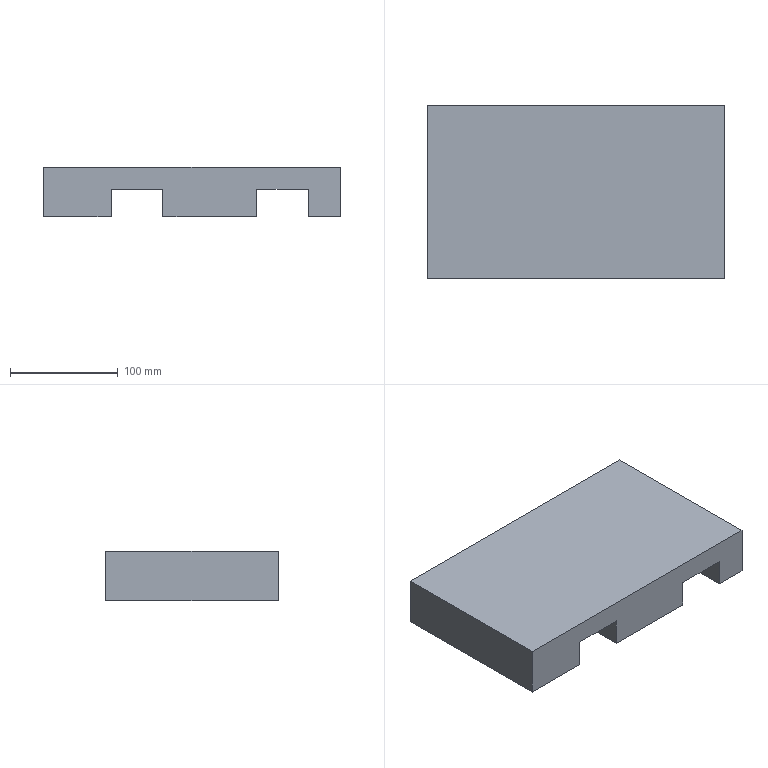Part | 1 solid | 14 faces | box 275.4 x 160 x 46 mm | volume 1635264 mm3 | plane 14
STEP:
#1=CARTESIAN_POINT('',(0.,0.,0.));
#2=DIRECTION('',(0.,0.,1.));
#3=DIRECTION('',(1.,0.,0.));
#4=AXIS2_PLACEMENT_3D('',#1,#2,#3);
#5=CARTESIAN_POINT('',(-116.3,226.5,-322.55));
#6=VERTEX_POINT('',#5);
#7=CARTESIAN_POINT('',(-116.3,226.5,-276.55));
#8=VERTEX_POINT('',#7);
#9=CARTESIAN_POINT('',(-116.3,226.5,-306.55));
#10=DIRECTION('',(0.,0.,1.));
#11=VECTOR('',#10,1.);
#12=LINE('',#9,#11);
#13=CARTESIAN_POINT('',(-116.3,386.5,-306.55));
#14=DIRECTION('',(1.,0.,0.));
#15=DIRECTION('',(0.,0.,-1.));
#16=AXIS2_PLACEMENT_3D('',#13,#14,#15);
#17=PLANE('',#16);
#18=CARTESIAN_POINT('',(0.,-160.));
#19=DIRECTION('',(-1.,0.));
#20=VECTOR('',#19,1.);
#21=LINE('',#18,#20);
#22=(GEOMETRIC_REPRESENTATION_CONTEXT(2)PARAMETRIC_REPRESENTATION_CONTEXT()REPRESENTATION_CONTEXT('',''));
#23=DEFINITIONAL_REPRESENTATION('',(#21),#22);
#24=PCURVE('',#17,#23);
#25=CARTESIAN_POINT('',(-287.5,226.5,-306.55));
#26=DIRECTION('',(0.,1.,0.));
#27=DIRECTION('',(0.,0.,-1.));
#28=AXIS2_PLACEMENT_3D('',#25,#26,#27);
#29=PLANE('',#28);
#30=CARTESIAN_POINT('',(0.,-171.2));
#31=DIRECTION('',(-1.,0.));
#32=VECTOR('',#31,1.);
#33=LINE('',#30,#32);
#34=(GEOMETRIC_REPRESENTATION_CONTEXT(2)PARAMETRIC_REPRESENTATION_CONTEXT()REPRESENTATION_CONTEXT('',''));
#35=DEFINITIONAL_REPRESENTATION('',(#33),#34);
#36=PCURVE('',#29,#35);
#37=SURFACE_CURVE('',#12,(#24,#36),.PCURVE_S1.);
#38=EDGE_CURVE('',#6,#8,#37,.T.);
#39=ORIENTED_EDGE('',*,*,#38,.F.);
#40=CARTESIAN_POINT('',(-116.3,386.5,-322.55));
#41=VERTEX_POINT('',#40);
#42=CARTESIAN_POINT('',(-116.3,386.5,-322.55));
#43=DIRECTION('',(0.,-1.,0.));
#44=VECTOR('',#43,1.);
#45=LINE('',#42,#44);
#46=CARTESIAN_POINT('',(16.,0.));
#47=DIRECTION('',(0.,-1.));
#48=VECTOR('',#47,1.);
#49=LINE('',#46,#48);
#50=(GEOMETRIC_REPRESENTATION_CONTEXT(2)PARAMETRIC_REPRESENTATION_CONTEXT()REPRESENTATION_CONTEXT('',''));
#51=DEFINITIONAL_REPRESENTATION('',(#49),#50);
#52=PCURVE('',#17,#51);
#53=CARTESIAN_POINT('',(-384.03,386.5,-322.55));
#54=DIRECTION('',(0.,0.,1.));
#55=DIRECTION('',(1.,0.,0.));
#56=AXIS2_PLACEMENT_3D('',#53,#54,#55);
#57=PLANE('',#56);
#58=CARTESIAN_POINT('',(267.73,0.));
#59=DIRECTION('',(0.,-1.));
#60=VECTOR('',#59,1.);
#61=LINE('',#58,#60);
#62=(GEOMETRIC_REPRESENTATION_CONTEXT(2)PARAMETRIC_REPRESENTATION_CONTEXT()REPRESENTATION_CONTEXT('',''));
#63=DEFINITIONAL_REPRESENTATION('',(#61),#62);
#64=PCURVE('',#57,#63);
#65=SURFACE_CURVE('',#45,(#52,#64),.PCURVE_S1.);
#66=EDGE_CURVE('',#41,#6,#65,.T.);
#67=ORIENTED_EDGE('',*,*,#66,.F.);
#68=CARTESIAN_POINT('',(-116.3,386.5,-276.55));
#69=VERTEX_POINT('',#68);
#70=CARTESIAN_POINT('',(-116.3,386.5,-306.55));
#71=DIRECTION('',(0.,0.,1.));
#72=VECTOR('',#71,1.);
#73=LINE('',#70,#72);
#74=CARTESIAN_POINT('',(0.,0.));
#75=DIRECTION('',(-1.,0.));
#76=VECTOR('',#75,1.);
#77=LINE('',#74,#76);
#78=(GEOMETRIC_REPRESENTATION_CONTEXT(2)PARAMETRIC_REPRESENTATION_CONTEXT()REPRESENTATION_CONTEXT('',''));
#79=DEFINITIONAL_REPRESENTATION('',(#77),#78);
#80=PCURVE('',#17,#79);
#81=CARTESIAN_POINT('',(-287.5,386.5,-306.55));
#82=DIRECTION('',(0.,1.,0.));
#83=DIRECTION('',(0.,0.,-1.));
#84=AXIS2_PLACEMENT_3D('',#81,#82,#83);
#85=PLANE('',#84);
#86=CARTESIAN_POINT('',(0.,-171.2));
#87=DIRECTION('',(-1.,0.));
#88=VECTOR('',#87,1.);
#89=LINE('',#86,#88);
#90=(GEOMETRIC_REPRESENTATION_CONTEXT(2)PARAMETRIC_REPRESENTATION_CONTEXT()REPRESENTATION_CONTEXT('',''));
#91=DEFINITIONAL_REPRESENTATION('',(#89),#90);
#92=PCURVE('',#85,#91);
#93=SURFACE_CURVE('',#73,(#80,#92),.PCURVE_S1.);
#94=EDGE_CURVE('',#41,#69,#93,.T.);
#95=ORIENTED_EDGE('',*,*,#94,.T.);
#96=CARTESIAN_POINT('',(-116.3,386.5,-276.55));
#97=DIRECTION('',(0.,-1.,0.));
#98=VECTOR('',#97,1.);
#99=LINE('',#96,#98);
#100=CARTESIAN_POINT('',(-30.,0.));
#101=DIRECTION('',(0.,-1.));
#102=VECTOR('',#101,1.);
#103=LINE('',#100,#102);
#104=(GEOMETRIC_REPRESENTATION_CONTEXT(2)PARAMETRIC_REPRESENTATION_CONTEXT()REPRESENTATION_CONTEXT('',''));
#105=DEFINITIONAL_REPRESENTATION('',(#103),#104);
#106=PCURVE('',#17,#105);
#107=CARTESIAN_POINT('',(-287.5,386.5,-276.55));
#108=DIRECTION('',(0.,0.,-1.));
#109=DIRECTION('',(-1.,0.,0.));
#110=AXIS2_PLACEMENT_3D('',#107,#108,#109);
#111=PLANE('',#110);
#112=CARTESIAN_POINT('',(-171.2,0.));
#113=DIRECTION('',(0.,-1.));
#114=VECTOR('',#113,1.);
#115=LINE('',#112,#114);
#116=(GEOMETRIC_REPRESENTATION_CONTEXT(2)PARAMETRIC_REPRESENTATION_CONTEXT()REPRESENTATION_CONTEXT('',''));
#117=DEFINITIONAL_REPRESENTATION('',(#115),#116);
#118=PCURVE('',#111,#117);
#119=SURFACE_CURVE('',#99,(#106,#118),.PCURVE_S1.);
#120=EDGE_CURVE('',#69,#8,#119,.T.);
#121=ORIENTED_EDGE('',*,*,#120,.T.);
#122=EDGE_LOOP('',(#39,#67,#95,#121));
#123=FACE_BOUND('',#122,.T.);
#124=ADVANCED_FACE('',(#123),#17,.T.);
#125=CARTESIAN_POINT('',(-391.7,226.5,-276.55));
#126=VERTEX_POINT('',#125);
#127=CARTESIAN_POINT('',(-287.5,226.5,-276.55));
#128=DIRECTION('',(1.,0.,0.));
#129=VECTOR('',#128,1.);
#130=LINE('',#127,#129);
#131=CARTESIAN_POINT('',(0.,-160.));
#132=DIRECTION('',(-1.,0.));
#133=VECTOR('',#132,1.);
#134=LINE('',#131,#133);
#135=(GEOMETRIC_REPRESENTATION_CONTEXT(2)PARAMETRIC_REPRESENTATION_CONTEXT()REPRESENTATION_CONTEXT('',''));
#136=DEFINITIONAL_REPRESENTATION('',(#134),#135);
#137=PCURVE('',#111,#136);
#138=CARTESIAN_POINT('',(-30.,0.));
#139=DIRECTION('',(0.,-1.));
#140=VECTOR('',#139,1.);
#141=LINE('',#138,#140);
#142=(GEOMETRIC_REPRESENTATION_CONTEXT(2)PARAMETRIC_REPRESENTATION_CONTEXT()REPRESENTATION_CONTEXT('',''));
#143=DEFINITIONAL_REPRESENTATION('',(#141),#142);
#144=PCURVE('',#29,#143);
#145=SURFACE_CURVE('',#130,(#137,#144),.PCURVE_S1.);
#146=EDGE_CURVE('',#126,#8,#145,.T.);
#147=ORIENTED_EDGE('',*,*,#146,.T.);
#148=ORIENTED_EDGE('',*,*,#120,.F.);
#149=CARTESIAN_POINT('',(-391.7,386.5,-276.55));
#150=VERTEX_POINT('',#149);
#151=CARTESIAN_POINT('',(-287.5,386.5,-276.55));
#152=DIRECTION('',(1.,0.,0.));
#153=VECTOR('',#152,1.);
#154=LINE('',#151,#153);
#155=CARTESIAN_POINT('',(0.,0.));
#156=DIRECTION('',(-1.,0.));
#157=VECTOR('',#156,1.);
#158=LINE('',#155,#157);
#159=(GEOMETRIC_REPRESENTATION_CONTEXT(2)PARAMETRIC_REPRESENTATION_CONTEXT()REPRESENTATION_CONTEXT('',''));
#160=DEFINITIONAL_REPRESENTATION('',(#158),#159);
#161=PCURVE('',#111,#160);
#162=CARTESIAN_POINT('',(-30.,0.));
#163=DIRECTION('',(0.,-1.));
#164=VECTOR('',#163,1.);
#165=LINE('',#162,#164);
#166=(GEOMETRIC_REPRESENTATION_CONTEXT(2)PARAMETRIC_REPRESENTATION_CONTEXT()REPRESENTATION_CONTEXT('',''));
#167=DEFINITIONAL_REPRESENTATION('',(#165),#166);
#168=PCURVE('',#85,#167);
#169=SURFACE_CURVE('',#154,(#161,#168),.PCURVE_S1.);
#170=EDGE_CURVE('',#150,#69,#169,.T.);
#171=ORIENTED_EDGE('',*,*,#170,.F.);
#172=CARTESIAN_POINT('',(-391.7,386.5,-276.55));
#173=DIRECTION('',(0.,-1.,0.));
#174=VECTOR('',#173,1.);
#175=LINE('',#172,#174);
#176=CARTESIAN_POINT('',(104.2,0.));
#177=DIRECTION('',(0.,-1.));
#178=VECTOR('',#177,1.);
#179=LINE('',#176,#178);
#180=(GEOMETRIC_REPRESENTATION_CONTEXT(2)PARAMETRIC_REPRESENTATION_CONTEXT()REPRESENTATION_CONTEXT('',''));
#181=DEFINITIONAL_REPRESENTATION('',(#179),#180);
#182=PCURVE('',#111,#181);
#183=CARTESIAN_POINT('',(-391.7,386.5,-306.55));
#184=DIRECTION('',(-1.,0.,0.));
#185=DIRECTION('',(0.,0.,1.));
#186=AXIS2_PLACEMENT_3D('',#183,#184,#185);
#187=PLANE('',#186);
#188=CARTESIAN_POINT('',(30.,0.));
#189=DIRECTION('',(0.,-1.));
#190=VECTOR('',#189,1.);
#191=LINE('',#188,#190);
#192=(GEOMETRIC_REPRESENTATION_CONTEXT(2)PARAMETRIC_REPRESENTATION_CONTEXT()REPRESENTATION_CONTEXT('',''));
#193=DEFINITIONAL_REPRESENTATION('',(#191),#192);
#194=PCURVE('',#187,#193);
#195=SURFACE_CURVE('',#175,(#182,#194),.PCURVE_S1.);
#196=EDGE_CURVE('',#150,#126,#195,.T.);
#197=ORIENTED_EDGE('',*,*,#196,.T.);
#198=EDGE_LOOP('',(#147,#148,#171,#197));
#199=FACE_BOUND('',#198,.T.);
#200=ADVANCED_FACE('',(#199),#111,.F.);
#201=CARTESIAN_POINT('',(-391.7,226.5,-322.55));
#202=VERTEX_POINT('',#201);
#203=CARTESIAN_POINT('',(-391.7,226.5,-306.55));
#204=DIRECTION('',(0.,0.,-1.));
#205=VECTOR('',#204,1.);
#206=LINE('',#203,#205);
#207=CARTESIAN_POINT('',(0.,-160.));
#208=DIRECTION('',(-1.,0.));
#209=VECTOR('',#208,1.);
#210=LINE('',#207,#209);
#211=(GEOMETRIC_REPRESENTATION_CONTEXT(2)PARAMETRIC_REPRESENTATION_CONTEXT()REPRESENTATION_CONTEXT('',''));
#212=DEFINITIONAL_REPRESENTATION('',(#210),#211);
#213=PCURVE('',#187,#212);
#214=CARTESIAN_POINT('',(0.,104.2));
#215=DIRECTION('',(1.,0.));
#216=VECTOR('',#215,1.);
#217=LINE('',#214,#216);
#218=(GEOMETRIC_REPRESENTATION_CONTEXT(2)PARAMETRIC_REPRESENTATION_CONTEXT()REPRESENTATION_CONTEXT('',''));
#219=DEFINITIONAL_REPRESENTATION('',(#217),#218);
#220=PCURVE('',#29,#219);
#221=SURFACE_CURVE('',#206,(#213,#220),.PCURVE_S1.);
#222=EDGE_CURVE('',#126,#202,#221,.T.);
#223=ORIENTED_EDGE('',*,*,#222,.F.);
#224=ORIENTED_EDGE('',*,*,#196,.F.);
#225=CARTESIAN_POINT('',(-391.7,386.5,-322.55));
#226=VERTEX_POINT('',#225);
#227=CARTESIAN_POINT('',(-391.7,386.5,-306.55));
#228=DIRECTION('',(0.,0.,-1.));
#229=VECTOR('',#228,1.);
#230=LINE('',#227,#229);
#231=CARTESIAN_POINT('',(0.,0.));
#232=DIRECTION('',(-1.,0.));
#233=VECTOR('',#232,1.);
#234=LINE('',#231,#233);
#235=(GEOMETRIC_REPRESENTATION_CONTEXT(2)PARAMETRIC_REPRESENTATION_CONTEXT()REPRESENTATION_CONTEXT('',''));
#236=DEFINITIONAL_REPRESENTATION('',(#234),#235);
#237=PCURVE('',#187,#236);
#238=CARTESIAN_POINT('',(0.,104.2));
#239=DIRECTION('',(1.,0.));
#240=VECTOR('',#239,1.);
#241=LINE('',#238,#240);
#242=(GEOMETRIC_REPRESENTATION_CONTEXT(2)PARAMETRIC_REPRESENTATION_CONTEXT()REPRESENTATION_CONTEXT('',''));
#243=DEFINITIONAL_REPRESENTATION('',(#241),#242);
#244=PCURVE('',#85,#243);
#245=SURFACE_CURVE('',#230,(#237,#244),.PCURVE_S1.);
#246=EDGE_CURVE('',#150,#226,#245,.T.);
#247=ORIENTED_EDGE('',*,*,#246,.T.);
#248=CARTESIAN_POINT('',(-391.7,386.5,-322.55));
#249=DIRECTION('',(0.,-1.,0.));
#250=VECTOR('',#249,1.);
#251=LINE('',#248,#250);
#252=CARTESIAN_POINT('',(-16.,0.));
#253=DIRECTION('',(0.,-1.));
#254=VECTOR('',#253,1.);
#255=LINE('',#252,#254);
#256=(GEOMETRIC_REPRESENTATION_CONTEXT(2)PARAMETRIC_REPRESENTATION_CONTEXT()REPRESENTATION_CONTEXT('',''));
#257=DEFINITIONAL_REPRESENTATION('',(#255),#256);
#258=PCURVE('',#187,#257);
#259=CARTESIAN_POINT('',(-384.03,386.5,-322.55));
#260=DIRECTION('',(0.,0.,1.));
#261=DIRECTION('',(1.,0.,0.));
#262=AXIS2_PLACEMENT_3D('',#259,#260,#261);
#263=PLANE('',#262);
#264=CARTESIAN_POINT('',(-7.67,0.));
#265=DIRECTION('',(0.,-1.));
#266=VECTOR('',#265,1.);
#267=LINE('',#264,#266);
#268=(GEOMETRIC_REPRESENTATION_CONTEXT(2)PARAMETRIC_REPRESENTATION_CONTEXT()REPRESENTATION_CONTEXT('',''));
#269=DEFINITIONAL_REPRESENTATION('',(#267),#268);
#270=PCURVE('',#263,#269);
#271=SURFACE_CURVE('',#251,(#258,#270),.PCURVE_S1.);
#272=EDGE_CURVE('',#226,#202,#271,.T.);
#273=ORIENTED_EDGE('',*,*,#272,.T.);
#274=EDGE_LOOP('',(#223,#224,#247,#273));
#275=FACE_BOUND('',#274,.T.);
#276=ADVANCED_FACE('',(#275),#187,.T.);
#277=CARTESIAN_POINT('',(-329.,226.5,-322.55));
#278=VERTEX_POINT('',#277);
#279=CARTESIAN_POINT('',(-384.03,226.5,-322.55));
#280=DIRECTION('',(-1.,0.,0.));
#281=VECTOR('',#280,1.);
#282=LINE('',#279,#281);
#283=CARTESIAN_POINT('',(0.,-160.));
#284=DIRECTION('',(-1.,0.));
#285=VECTOR('',#284,1.);
#286=LINE('',#283,#285);
#287=(GEOMETRIC_REPRESENTATION_CONTEXT(2)PARAMETRIC_REPRESENTATION_CONTEXT()REPRESENTATION_CONTEXT('',''));
#288=DEFINITIONAL_REPRESENTATION('',(#286),#287);
#289=PCURVE('',#263,#288);
#290=CARTESIAN_POINT('',(16.,96.53));
#291=DIRECTION('',(0.,1.));
#292=VECTOR('',#291,1.);
#293=LINE('',#290,#292);
#294=(GEOMETRIC_REPRESENTATION_CONTEXT(2)PARAMETRIC_REPRESENTATION_CONTEXT()REPRESENTATION_CONTEXT('',''));
#295=DEFINITIONAL_REPRESENTATION('',(#293),#294);
#296=PCURVE('',#29,#295);
#297=SURFACE_CURVE('',#282,(#289,#296),.PCURVE_S1.);
#298=EDGE_CURVE('',#278,#202,#297,.T.);
#299=ORIENTED_EDGE('',*,*,#298,.T.);
#300=ORIENTED_EDGE('',*,*,#272,.F.);
#301=CARTESIAN_POINT('',(-329.,386.5,-322.55));
#302=VERTEX_POINT('',#301);
#303=CARTESIAN_POINT('',(-384.03,386.5,-322.55));
#304=DIRECTION('',(-1.,0.,0.));
#305=VECTOR('',#304,1.);
#306=LINE('',#303,#305);
#307=CARTESIAN_POINT('',(0.,0.));
#308=DIRECTION('',(-1.,0.));
#309=VECTOR('',#308,1.);
#310=LINE('',#307,#309);
#311=(GEOMETRIC_REPRESENTATION_CONTEXT(2)PARAMETRIC_REPRESENTATION_CONTEXT()REPRESENTATION_CONTEXT('',''));
#312=DEFINITIONAL_REPRESENTATION('',(#310),#311);
#313=PCURVE('',#263,#312);
#314=CARTESIAN_POINT('',(16.,96.53));
#315=DIRECTION('',(0.,1.));
#316=VECTOR('',#315,1.);
#317=LINE('',#314,#316);
#318=(GEOMETRIC_REPRESENTATION_CONTEXT(2)PARAMETRIC_REPRESENTATION_CONTEXT()REPRESENTATION_CONTEXT('',''));
#319=DEFINITIONAL_REPRESENTATION('',(#317),#318);
#320=PCURVE('',#85,#319);
#321=SURFACE_CURVE('',#306,(#313,#320),.PCURVE_S1.);
#322=EDGE_CURVE('',#302,#226,#321,.T.);
#323=ORIENTED_EDGE('',*,*,#322,.F.);
#324=CARTESIAN_POINT('',(-329.,386.5,-322.55));
#325=DIRECTION('',(0.,-1.,0.));
#326=VECTOR('',#325,1.);
#327=LINE('',#324,#326);
#328=CARTESIAN_POINT('',(55.03,0.));
#329=DIRECTION('',(0.,-1.));
#330=VECTOR('',#329,1.);
#331=LINE('',#328,#330);
#332=(GEOMETRIC_REPRESENTATION_CONTEXT(2)PARAMETRIC_REPRESENTATION_CONTEXT()REPRESENTATION_CONTEXT('',''));
#333=DEFINITIONAL_REPRESENTATION('',(#331),#332);
#334=PCURVE('',#263,#333);
#335=CARTESIAN_POINT('',(-329.,386.5,-306.55));
#336=DIRECTION('',(1.,0.,0.));
#337=DIRECTION('',(0.,0.,-1.));
#338=AXIS2_PLACEMENT_3D('',#335,#336,#337);
#339=PLANE('',#338);
#340=CARTESIAN_POINT('',(16.,0.));
#341=DIRECTION('',(0.,-1.));
#342=VECTOR('',#341,1.);
#343=LINE('',#340,#342);
#344=(GEOMETRIC_REPRESENTATION_CONTEXT(2)PARAMETRIC_REPRESENTATION_CONTEXT()REPRESENTATION_CONTEXT('',''));
#345=DEFINITIONAL_REPRESENTATION('',(#343),#344);
#346=PCURVE('',#339,#345);
#347=SURFACE_CURVE('',#327,(#334,#346),.PCURVE_S1.);
#348=EDGE_CURVE('',#302,#278,#347,.T.);
#349=ORIENTED_EDGE('',*,*,#348,.T.);
#350=EDGE_LOOP('',(#299,#300,#323,#349));
#351=FACE_BOUND('',#350,.T.);
#352=ADVANCED_FACE('',(#351),#263,.F.);
#353=CARTESIAN_POINT('',(-329.,226.5,-297.05));
#354=VERTEX_POINT('',#353);
#355=CARTESIAN_POINT('',(-329.,226.5,-306.55));
#356=DIRECTION('',(0.,0.,1.));
#357=VECTOR('',#356,1.);
#358=LINE('',#355,#357);
#359=CARTESIAN_POINT('',(0.,-160.));
#360=DIRECTION('',(-1.,0.));
#361=VECTOR('',#360,1.);
#362=LINE('',#359,#361);
#363=(GEOMETRIC_REPRESENTATION_CONTEXT(2)PARAMETRIC_REPRESENTATION_CONTEXT()REPRESENTATION_CONTEXT('',''));
#364=DEFINITIONAL_REPRESENTATION('',(#362),#363);
#365=PCURVE('',#339,#364);
#366=CARTESIAN_POINT('',(0.,41.5));
#367=DIRECTION('',(-1.,0.));
#368=VECTOR('',#367,1.);
#369=LINE('',#366,#368);
#370=(GEOMETRIC_REPRESENTATION_CONTEXT(2)PARAMETRIC_REPRESENTATION_CONTEXT()REPRESENTATION_CONTEXT('',''));
#371=DEFINITIONAL_REPRESENTATION('',(#369),#370);
#372=PCURVE('',#29,#371);
#373=SURFACE_CURVE('',#358,(#365,#372),.PCURVE_S1.);
#374=EDGE_CURVE('',#278,#354,#373,.T.);
#375=ORIENTED_EDGE('',*,*,#374,.F.);
#376=ORIENTED_EDGE('',*,*,#348,.F.);
#377=CARTESIAN_POINT('',(-329.,386.5,-297.05));
#378=VERTEX_POINT('',#377);
#379=CARTESIAN_POINT('',(-329.,386.5,-306.55));
#380=DIRECTION('',(0.,0.,1.));
#381=VECTOR('',#380,1.);
#382=LINE('',#379,#381);
#383=CARTESIAN_POINT('',(0.,0.));
#384=DIRECTION('',(-1.,0.));
#385=VECTOR('',#384,1.);
#386=LINE('',#383,#385);
#387=(GEOMETRIC_REPRESENTATION_CONTEXT(2)PARAMETRIC_REPRESENTATION_CONTEXT()REPRESENTATION_CONTEXT('',''));
#388=DEFINITIONAL_REPRESENTATION('',(#386),#387);
#389=PCURVE('',#339,#388);
#390=CARTESIAN_POINT('',(0.,41.5));
#391=DIRECTION('',(-1.,0.));
#392=VECTOR('',#391,1.);
#393=LINE('',#390,#392);
#394=(GEOMETRIC_REPRESENTATION_CONTEXT(2)PARAMETRIC_REPRESENTATION_CONTEXT()REPRESENTATION_CONTEXT('',''));
#395=DEFINITIONAL_REPRESENTATION('',(#393),#394);
#396=PCURVE('',#85,#395);
#397=SURFACE_CURVE('',#382,(#389,#396),.PCURVE_S1.);
#398=EDGE_CURVE('',#302,#378,#397,.T.);
#399=ORIENTED_EDGE('',*,*,#398,.T.);
#400=CARTESIAN_POINT('',(-329.,386.5,-297.05));
#401=DIRECTION('',(0.,-1.,0.));
#402=VECTOR('',#401,1.);
#403=LINE('',#400,#402);
#404=CARTESIAN_POINT('',(-9.5,0.));
#405=DIRECTION('',(0.,-1.));
#406=VECTOR('',#405,1.);
#407=LINE('',#404,#406);
#408=(GEOMETRIC_REPRESENTATION_CONTEXT(2)PARAMETRIC_REPRESENTATION_CONTEXT()REPRESENTATION_CONTEXT('',''));
#409=DEFINITIONAL_REPRESENTATION('',(#407),#408);
#410=PCURVE('',#339,#409);
#411=CARTESIAN_POINT('',(-287.5,386.5,-297.05));
#412=DIRECTION('',(0.,0.,-1.));
#413=DIRECTION('',(-1.,0.,0.));
#414=AXIS2_PLACEMENT_3D('',#411,#412,#413);
#415=PLANE('',#414);
#416=CARTESIAN_POINT('',(41.5,0.));
#417=DIRECTION('',(0.,-1.));
#418=VECTOR('',#417,1.);
#419=LINE('',#416,#418);
#420=(GEOMETRIC_REPRESENTATION_CONTEXT(2)PARAMETRIC_REPRESENTATION_CONTEXT()REPRESENTATION_CONTEXT('',''));
#421=DEFINITIONAL_REPRESENTATION('',(#419),#420);
#422=PCURVE('',#415,#421);
#423=SURFACE_CURVE('',#403,(#410,#422),.PCURVE_S1.);
#424=EDGE_CURVE('',#378,#354,#423,.T.);
#425=ORIENTED_EDGE('',*,*,#424,.T.);
#426=EDGE_LOOP('',(#375,#376,#399,#425));
#427=FACE_BOUND('',#426,.T.);
#428=ADVANCED_FACE('',(#427),#339,.T.);
#429=CARTESIAN_POINT('',(-281.,226.5,-297.05));
#430=VERTEX_POINT('',#429);
#431=CARTESIAN_POINT('',(-287.5,226.5,-297.05));
#432=DIRECTION('',(1.,0.,0.));
#433=VECTOR('',#432,1.);
#434=LINE('',#431,#433);
#435=CARTESIAN_POINT('',(0.,-160.));
#436=DIRECTION('',(-1.,0.));
#437=VECTOR('',#436,1.);
#438=LINE('',#435,#437);
#439=(GEOMETRIC_REPRESENTATION_CONTEXT(2)PARAMETRIC_REPRESENTATION_CONTEXT()REPRESENTATION_CONTEXT('',''));
#440=DEFINITIONAL_REPRESENTATION('',(#438),#439);
#441=PCURVE('',#415,#440);
#442=CARTESIAN_POINT('',(-9.5,0.));
#443=DIRECTION('',(0.,-1.));
#444=VECTOR('',#443,1.);
#445=LINE('',#442,#444);
#446=(GEOMETRIC_REPRESENTATION_CONTEXT(2)PARAMETRIC_REPRESENTATION_CONTEXT()REPRESENTATION_CONTEXT('',''));
#447=DEFINITIONAL_REPRESENTATION('',(#445),#446);
#448=PCURVE('',#29,#447);
#449=SURFACE_CURVE('',#434,(#441,#448),.PCURVE_S1.);
#450=EDGE_CURVE('',#354,#430,#449,.T.);
#451=ORIENTED_EDGE('',*,*,#450,.F.);
#452=ORIENTED_EDGE('',*,*,#424,.F.);
#453=CARTESIAN_POINT('',(-281.,386.5,-297.05));
#454=VERTEX_POINT('',#453);
#455=CARTESIAN_POINT('',(-287.5,386.5,-297.05));
#456=DIRECTION('',(1.,0.,0.));
#457=VECTOR('',#456,1.);
#458=LINE('',#455,#457);
#459=CARTESIAN_POINT('',(0.,0.));
#460=DIRECTION('',(-1.,0.));
#461=VECTOR('',#460,1.);
#462=LINE('',#459,#461);
#463=(GEOMETRIC_REPRESENTATION_CONTEXT(2)PARAMETRIC_REPRESENTATION_CONTEXT()REPRESENTATION_CONTEXT('',''));
#464=DEFINITIONAL_REPRESENTATION('',(#462),#463);
#465=PCURVE('',#415,#464);
#466=CARTESIAN_POINT('',(-9.5,0.));
#467=DIRECTION('',(0.,-1.));
#468=VECTOR('',#467,1.);
#469=LINE('',#466,#468);
#470=(GEOMETRIC_REPRESENTATION_CONTEXT(2)PARAMETRIC_REPRESENTATION_CONTEXT()REPRESENTATION_CONTEXT('',''));
#471=DEFINITIONAL_REPRESENTATION('',(#469),#470);
#472=PCURVE('',#85,#471);
#473=SURFACE_CURVE('',#458,(#465,#472),.PCURVE_S1.);
#474=EDGE_CURVE('',#378,#454,#473,.T.);
#475=ORIENTED_EDGE('',*,*,#474,.T.);
#476=CARTESIAN_POINT('',(-281.,386.5,-297.05));
#477=DIRECTION('',(0.,-1.,0.));
#478=VECTOR('',#477,1.);
#479=LINE('',#476,#478);
#480=CARTESIAN_POINT('',(-6.5,0.));
#481=DIRECTION('',(0.,-1.));
#482=VECTOR('',#481,1.);
#483=LINE('',#480,#482);
#484=(GEOMETRIC_REPRESENTATION_CONTEXT(2)PARAMETRIC_REPRESENTATION_CONTEXT()REPRESENTATION_CONTEXT('',''));
#485=DEFINITIONAL_REPRESENTATION('',(#483),#484);
#486=PCURVE('',#415,#485);
#487=CARTESIAN_POINT('',(-281.,386.5,-306.55));
#488=DIRECTION('',(-1.,0.,0.));
#489=DIRECTION('',(0.,0.,1.));
#490=AXIS2_PLACEMENT_3D('',#487,#488,#489);
#491=PLANE('',#490);
#492=CARTESIAN_POINT('',(9.5,0.));
#493=DIRECTION('',(0.,-1.));
#494=VECTOR('',#493,1.);
#495=LINE('',#492,#494);
#496=(GEOMETRIC_REPRESENTATION_CONTEXT(2)PARAMETRIC_REPRESENTATION_CONTEXT()REPRESENTATION_CONTEXT('',''));
#497=DEFINITIONAL_REPRESENTATION('',(#495),#496);
#498=PCURVE('',#491,#497);
#499=SURFACE_CURVE('',#479,(#486,#498),.PCURVE_S1.);
#500=EDGE_CURVE('',#454,#430,#499,.T.);
#501=ORIENTED_EDGE('',*,*,#500,.T.);
#502=EDGE_LOOP('',(#451,#452,#475,#501));
#503=FACE_BOUND('',#502,.T.);
#504=ADVANCED_FACE('',(#503),#415,.T.);
#505=CARTESIAN_POINT('',(-281.,226.5,-322.55));
#506=VERTEX_POINT('',#505);
#507=CARTESIAN_POINT('',(-281.,226.5,-306.55));
#508=DIRECTION('',(0.,0.,-1.));
#509=VECTOR('',#508,1.);
#510=LINE('',#507,#509);
#511=CARTESIAN_POINT('',(0.,-160.));
#512=DIRECTION('',(-1.,0.));
#513=VECTOR('',#512,1.);
#514=LINE('',#511,#513);
#515=(GEOMETRIC_REPRESENTATION_CONTEXT(2)PARAMETRIC_REPRESENTATION_CONTEXT()REPRESENTATION_CONTEXT('',''));
#516=DEFINITIONAL_REPRESENTATION('',(#514),#515);
#517=PCURVE('',#491,#516);
#518=CARTESIAN_POINT('',(0.,-6.5));
#519=DIRECTION('',(1.,0.));
#520=VECTOR('',#519,1.);
#521=LINE('',#518,#520);
#522=(GEOMETRIC_REPRESENTATION_CONTEXT(2)PARAMETRIC_REPRESENTATION_CONTEXT()REPRESENTATION_CONTEXT('',''));
#523=DEFINITIONAL_REPRESENTATION('',(#521),#522);
#524=PCURVE('',#29,#523);
#525=SURFACE_CURVE('',#510,(#517,#524),.PCURVE_S1.);
#526=EDGE_CURVE('',#430,#506,#525,.T.);
#527=ORIENTED_EDGE('',*,*,#526,.F.);
#528=ORIENTED_EDGE('',*,*,#500,.F.);
#529=CARTESIAN_POINT('',(-281.,386.5,-322.55));
#530=VERTEX_POINT('',#529);
#531=CARTESIAN_POINT('',(-281.,386.5,-306.55));
#532=DIRECTION('',(0.,0.,-1.));
#533=VECTOR('',#532,1.);
#534=LINE('',#531,#533);
#535=CARTESIAN_POINT('',(0.,0.));
#536=DIRECTION('',(-1.,0.));
#537=VECTOR('',#536,1.);
#538=LINE('',#535,#537);
#539=(GEOMETRIC_REPRESENTATION_CONTEXT(2)PARAMETRIC_REPRESENTATION_CONTEXT()REPRESENTATION_CONTEXT('',''));
#540=DEFINITIONAL_REPRESENTATION('',(#538),#539);
#541=PCURVE('',#491,#540);
#542=CARTESIAN_POINT('',(0.,-6.5));
#543=DIRECTION('',(1.,0.));
#544=VECTOR('',#543,1.);
#545=LINE('',#542,#544);
#546=(GEOMETRIC_REPRESENTATION_CONTEXT(2)PARAMETRIC_REPRESENTATION_CONTEXT()REPRESENTATION_CONTEXT('',''));
#547=DEFINITIONAL_REPRESENTATION('',(#545),#546);
#548=PCURVE('',#85,#547);
#549=SURFACE_CURVE('',#534,(#541,#548),.PCURVE_S1.);
#550=EDGE_CURVE('',#454,#530,#549,.T.);
#551=ORIENTED_EDGE('',*,*,#550,.T.);
#552=CARTESIAN_POINT('',(-281.,386.5,-322.55));
#553=DIRECTION('',(0.,-1.,0.));
#554=VECTOR('',#553,1.);
#555=LINE('',#552,#554);
#556=CARTESIAN_POINT('',(-16.,0.));
#557=DIRECTION('',(0.,-1.));
#558=VECTOR('',#557,1.);
#559=LINE('',#556,#558);
#560=(GEOMETRIC_REPRESENTATION_CONTEXT(2)PARAMETRIC_REPRESENTATION_CONTEXT()REPRESENTATION_CONTEXT('',''));
#561=DEFINITIONAL_REPRESENTATION('',(#559),#560);
#562=PCURVE('',#491,#561);
#563=CARTESIAN_POINT('',(-384.03,386.5,-322.55));
#564=DIRECTION('',(0.,0.,1.));
#565=DIRECTION('',(1.,0.,0.));
#566=AXIS2_PLACEMENT_3D('',#563,#564,#565);
#567=PLANE('',#566);
#568=CARTESIAN_POINT('',(103.03,0.));
#569=DIRECTION('',(0.,-1.));
#570=VECTOR('',#569,1.);
#571=LINE('',#568,#570);
#572=(GEOMETRIC_REPRESENTATION_CONTEXT(2)PARAMETRIC_REPRESENTATION_CONTEXT()REPRESENTATION_CONTEXT('',''));
#573=DEFINITIONAL_REPRESENTATION('',(#571),#572);
#574=PCURVE('',#567,#573);
#575=SURFACE_CURVE('',#555,(#562,#574),.PCURVE_S1.);
#576=EDGE_CURVE('',#530,#506,#575,.T.);
#577=ORIENTED_EDGE('',*,*,#576,.T.);
#578=EDGE_LOOP('',(#527,#528,#551,#577));
#579=FACE_BOUND('',#578,.T.);
#580=ADVANCED_FACE('',(#579),#491,.T.);
#581=CARTESIAN_POINT('',(-194.,226.5,-322.55));
#582=VERTEX_POINT('',#581);
#583=CARTESIAN_POINT('',(-384.03,226.5,-322.55));
#584=DIRECTION('',(-1.,0.,0.));
#585=VECTOR('',#584,1.);
#586=LINE('',#583,#585);
#587=CARTESIAN_POINT('',(0.,-160.));
#588=DIRECTION('',(-1.,0.));
#589=VECTOR('',#588,1.);
#590=LINE('',#587,#589);
#591=(GEOMETRIC_REPRESENTATION_CONTEXT(2)PARAMETRIC_REPRESENTATION_CONTEXT()REPRESENTATION_CONTEXT('',''));
#592=DEFINITIONAL_REPRESENTATION('',(#590),#591);
#593=PCURVE('',#567,#592);
#594=CARTESIAN_POINT('',(16.,96.53));
#595=DIRECTION('',(0.,1.));
#596=VECTOR('',#595,1.);
#597=LINE('',#594,#596);
#598=(GEOMETRIC_REPRESENTATION_CONTEXT(2)PARAMETRIC_REPRESENTATION_CONTEXT()REPRESENTATION_CONTEXT('',''));
#599=DEFINITIONAL_REPRESENTATION('',(#597),#598);
#600=PCURVE('',#29,#599);
#601=SURFACE_CURVE('',#586,(#593,#600),.PCURVE_S1.);
#602=EDGE_CURVE('',#582,#506,#601,.T.);
#603=ORIENTED_EDGE('',*,*,#602,.T.);
#604=ORIENTED_EDGE('',*,*,#576,.F.);
#605=CARTESIAN_POINT('',(-194.,386.5,-322.55));
#606=VERTEX_POINT('',#605);
#607=CARTESIAN_POINT('',(-384.03,386.5,-322.55));
#608=DIRECTION('',(-1.,0.,0.));
#609=VECTOR('',#608,1.);
#610=LINE('',#607,#609);
#611=CARTESIAN_POINT('',(0.,0.));
#612=DIRECTION('',(-1.,0.));
#613=VECTOR('',#612,1.);
#614=LINE('',#611,#613);
#615=(GEOMETRIC_REPRESENTATION_CONTEXT(2)PARAMETRIC_REPRESENTATION_CONTEXT()REPRESENTATION_CONTEXT('',''));
#616=DEFINITIONAL_REPRESENTATION('',(#614),#615);
#617=PCURVE('',#567,#616);
#618=CARTESIAN_POINT('',(16.,96.53));
#619=DIRECTION('',(0.,1.));
#620=VECTOR('',#619,1.);
#621=LINE('',#618,#620);
#622=(GEOMETRIC_REPRESENTATION_CONTEXT(2)PARAMETRIC_REPRESENTATION_CONTEXT()REPRESENTATION_CONTEXT('',''));
#623=DEFINITIONAL_REPRESENTATION('',(#621),#622);
#624=PCURVE('',#85,#623);
#625=SURFACE_CURVE('',#610,(#617,#624),.PCURVE_S1.);
#626=EDGE_CURVE('',#606,#530,#625,.T.);
#627=ORIENTED_EDGE('',*,*,#626,.F.);
#628=CARTESIAN_POINT('',(-194.,386.5,-322.55));
#629=DIRECTION('',(0.,-1.,0.));
#630=VECTOR('',#629,1.);
#631=LINE('',#628,#630);
#632=CARTESIAN_POINT('',(190.03,0.));
#633=DIRECTION('',(0.,-1.));
#634=VECTOR('',#633,1.);
#635=LINE('',#632,#634);
#636=(GEOMETRIC_REPRESENTATION_CONTEXT(2)PARAMETRIC_REPRESENTATION_CONTEXT()REPRESENTATION_CONTEXT('',''));
#637=DEFINITIONAL_REPRESENTATION('',(#635),#636);
#638=PCURVE('',#567,#637);
#639=CARTESIAN_POINT('',(-194.,386.5,-306.55));
#640=DIRECTION('',(-1.,0.,0.));
#641=DIRECTION('',(0.,0.,1.));
#642=AXIS2_PLACEMENT_3D('',#639,#640,#641);
#643=PLANE('',#642);
#644=CARTESIAN_POINT('',(-16.,0.));
#645=DIRECTION('',(0.,-1.));
#646=VECTOR('',#645,1.);
#647=LINE('',#644,#646);
#648=(GEOMETRIC_REPRESENTATION_CONTEXT(2)PARAMETRIC_REPRESENTATION_CONTEXT()REPRESENTATION_CONTEXT('',''));
#649=DEFINITIONAL_REPRESENTATION('',(#647),#648);
#650=PCURVE('',#643,#649);
#651=SURFACE_CURVE('',#631,(#638,#650),.PCURVE_S1.);
#652=EDGE_CURVE('',#606,#582,#651,.T.);
#653=ORIENTED_EDGE('',*,*,#652,.T.);
#654=EDGE_LOOP('',(#603,#604,#627,#653));
#655=FACE_BOUND('',#654,.T.);
#656=ADVANCED_FACE('',(#655),#567,.F.);
#657=CARTESIAN_POINT('',(-194.,226.5,-297.05));
#658=VERTEX_POINT('',#657);
#659=CARTESIAN_POINT('',(-194.,226.5,-306.55));
#660=DIRECTION('',(0.,0.,-1.));
#661=VECTOR('',#660,1.);
#662=LINE('',#659,#661);
#663=CARTESIAN_POINT('',(0.,-160.));
#664=DIRECTION('',(-1.,0.));
#665=VECTOR('',#664,1.);
#666=LINE('',#663,#665);
#667=(GEOMETRIC_REPRESENTATION_CONTEXT(2)PARAMETRIC_REPRESENTATION_CONTEXT()REPRESENTATION_CONTEXT('',''));
#668=DEFINITIONAL_REPRESENTATION('',(#666),#667);
#669=PCURVE('',#643,#668);
#670=CARTESIAN_POINT('',(0.,-93.5));
#671=DIRECTION('',(1.,0.));
#672=VECTOR('',#671,1.);
#673=LINE('',#670,#672);
#674=(GEOMETRIC_REPRESENTATION_CONTEXT(2)PARAMETRIC_REPRESENTATION_CONTEXT()REPRESENTATION_CONTEXT('',''));
#675=DEFINITIONAL_REPRESENTATION('',(#673),#674);
#676=PCURVE('',#29,#675);
#677=SURFACE_CURVE('',#662,(#669,#676),.PCURVE_S1.);
#678=EDGE_CURVE('',#658,#582,#677,.T.);
#679=ORIENTED_EDGE('',*,*,#678,.T.);
#680=ORIENTED_EDGE('',*,*,#652,.F.);
#681=CARTESIAN_POINT('',(-194.,386.5,-297.05));
#682=VERTEX_POINT('',#681);
#683=CARTESIAN_POINT('',(-194.,386.5,-306.55));
#684=DIRECTION('',(0.,0.,-1.));
#685=VECTOR('',#684,1.);
#686=LINE('',#683,#685);
#687=CARTESIAN_POINT('',(0.,0.));
#688=DIRECTION('',(-1.,0.));
#689=VECTOR('',#688,1.);
#690=LINE('',#687,#689);
#691=(GEOMETRIC_REPRESENTATION_CONTEXT(2)PARAMETRIC_REPRESENTATION_CONTEXT()REPRESENTATION_CONTEXT('',''));
#692=DEFINITIONAL_REPRESENTATION('',(#690),#691);
#693=PCURVE('',#643,#692);
#694=CARTESIAN_POINT('',(0.,-93.5));
#695=DIRECTION('',(1.,0.));
#696=VECTOR('',#695,1.);
#697=LINE('',#694,#696);
#698=(GEOMETRIC_REPRESENTATION_CONTEXT(2)PARAMETRIC_REPRESENTATION_CONTEXT()REPRESENTATION_CONTEXT('',''));
#699=DEFINITIONAL_REPRESENTATION('',(#697),#698);
#700=PCURVE('',#85,#699);
#701=SURFACE_CURVE('',#686,(#693,#700),.PCURVE_S1.);
#702=EDGE_CURVE('',#682,#606,#701,.T.);
#703=ORIENTED_EDGE('',*,*,#702,.F.);
#704=CARTESIAN_POINT('',(-194.,386.5,-297.05));
#705=DIRECTION('',(0.,-1.,0.));
#706=VECTOR('',#705,1.);
#707=LINE('',#704,#706);
#708=CARTESIAN_POINT('',(9.5,0.));
#709=DIRECTION('',(0.,-1.));
#710=VECTOR('',#709,1.);
#711=LINE('',#708,#710);
#712=(GEOMETRIC_REPRESENTATION_CONTEXT(2)PARAMETRIC_REPRESENTATION_CONTEXT()REPRESENTATION_CONTEXT('',''));
#713=DEFINITIONAL_REPRESENTATION('',(#711),#712);
#714=PCURVE('',#643,#713);
#715=CARTESIAN_POINT('',(-287.5,386.5,-297.05));
#716=DIRECTION('',(0.,0.,-1.));
#717=DIRECTION('',(-1.,0.,0.));
#718=AXIS2_PLACEMENT_3D('',#715,#716,#717);
#719=PLANE('',#718);
#720=CARTESIAN_POINT('',(-93.5,0.));
#721=DIRECTION('',(0.,-1.));
#722=VECTOR('',#721,1.);
#723=LINE('',#720,#722);
#724=(GEOMETRIC_REPRESENTATION_CONTEXT(2)PARAMETRIC_REPRESENTATION_CONTEXT()REPRESENTATION_CONTEXT('',''));
#725=DEFINITIONAL_REPRESENTATION('',(#723),#724);
#726=PCURVE('',#719,#725);
#727=SURFACE_CURVE('',#707,(#714,#726),.PCURVE_S1.);
#728=EDGE_CURVE('',#682,#658,#727,.T.);
#729=ORIENTED_EDGE('',*,*,#728,.T.);
#730=EDGE_LOOP('',(#679,#680,#703,#729));
#731=FACE_BOUND('',#730,.T.);
#732=ADVANCED_FACE('',(#731),#643,.F.);
#733=CARTESIAN_POINT('',(-146.,226.5,-297.05));
#734=VERTEX_POINT('',#733);
#735=CARTESIAN_POINT('',(-287.5,226.5,-297.05));
#736=DIRECTION('',(1.,0.,0.));
#737=VECTOR('',#736,1.);
#738=LINE('',#735,#737);
#739=CARTESIAN_POINT('',(0.,-160.));
#740=DIRECTION('',(-1.,0.));
#741=VECTOR('',#740,1.);
#742=LINE('',#739,#741);
#743=(GEOMETRIC_REPRESENTATION_CONTEXT(2)PARAMETRIC_REPRESENTATION_CONTEXT()REPRESENTATION_CONTEXT('',''));
#744=DEFINITIONAL_REPRESENTATION('',(#742),#743);
#745=PCURVE('',#719,#744);
#746=CARTESIAN_POINT('',(-9.5,0.));
#747=DIRECTION('',(0.,-1.));
#748=VECTOR('',#747,1.);
#749=LINE('',#746,#748);
#750=(GEOMETRIC_REPRESENTATION_CONTEXT(2)PARAMETRIC_REPRESENTATION_CONTEXT()REPRESENTATION_CONTEXT('',''));
#751=DEFINITIONAL_REPRESENTATION('',(#749),#750);
#752=PCURVE('',#29,#751);
#753=SURFACE_CURVE('',#738,(#745,#752),.PCURVE_S1.);
#754=EDGE_CURVE('',#658,#734,#753,.T.);
#755=ORIENTED_EDGE('',*,*,#754,.F.);
#756=ORIENTED_EDGE('',*,*,#728,.F.);
#757=CARTESIAN_POINT('',(-146.,386.5,-297.05));
#758=VERTEX_POINT('',#757);
#759=CARTESIAN_POINT('',(-287.5,386.5,-297.05));
#760=DIRECTION('',(1.,0.,0.));
#761=VECTOR('',#760,1.);
#762=LINE('',#759,#761);
#763=CARTESIAN_POINT('',(0.,0.));
#764=DIRECTION('',(-1.,0.));
#765=VECTOR('',#764,1.);
#766=LINE('',#763,#765);
#767=(GEOMETRIC_REPRESENTATION_CONTEXT(2)PARAMETRIC_REPRESENTATION_CONTEXT()REPRESENTATION_CONTEXT('',''));
#768=DEFINITIONAL_REPRESENTATION('',(#766),#767);
#769=PCURVE('',#719,#768);
#770=CARTESIAN_POINT('',(-9.5,0.));
#771=DIRECTION('',(0.,-1.));
#772=VECTOR('',#771,1.);
#773=LINE('',#770,#772);
#774=(GEOMETRIC_REPRESENTATION_CONTEXT(2)PARAMETRIC_REPRESENTATION_CONTEXT()REPRESENTATION_CONTEXT('',''));
#775=DEFINITIONAL_REPRESENTATION('',(#773),#774);
#776=PCURVE('',#85,#775);
#777=SURFACE_CURVE('',#762,(#769,#776),.PCURVE_S1.);
#778=EDGE_CURVE('',#682,#758,#777,.T.);
#779=ORIENTED_EDGE('',*,*,#778,.T.);
#780=CARTESIAN_POINT('',(-146.,386.5,-297.05));
#781=DIRECTION('',(0.,-1.,0.));
#782=VECTOR('',#781,1.);
#783=LINE('',#780,#782);
#784=CARTESIAN_POINT('',(-141.5,0.));
#785=DIRECTION('',(0.,-1.));
#786=VECTOR('',#785,1.);
#787=LINE('',#784,#786);
#788=(GEOMETRIC_REPRESENTATION_CONTEXT(2)PARAMETRIC_REPRESENTATION_CONTEXT()REPRESENTATION_CONTEXT('',''));
#789=DEFINITIONAL_REPRESENTATION('',(#787),#788);
#790=PCURVE('',#719,#789);
#791=CARTESIAN_POINT('',(-146.,386.5,-306.55));
#792=DIRECTION('',(-1.,0.,0.));
#793=DIRECTION('',(0.,0.,1.));
#794=AXIS2_PLACEMENT_3D('',#791,#792,#793);
#795=PLANE('',#794);
#796=CARTESIAN_POINT('',(9.5,0.));
#797=DIRECTION('',(0.,-1.));
#798=VECTOR('',#797,1.);
#799=LINE('',#796,#798);
#800=(GEOMETRIC_REPRESENTATION_CONTEXT(2)PARAMETRIC_REPRESENTATION_CONTEXT()REPRESENTATION_CONTEXT('',''));
#801=DEFINITIONAL_REPRESENTATION('',(#799),#800);
#802=PCURVE('',#795,#801);
#803=SURFACE_CURVE('',#783,(#790,#802),.PCURVE_S1.);
#804=EDGE_CURVE('',#758,#734,#803,.T.);
#805=ORIENTED_EDGE('',*,*,#804,.T.);
#806=EDGE_LOOP('',(#755,#756,#779,#805));
#807=FACE_BOUND('',#806,.T.);
#808=ADVANCED_FACE('',(#807),#719,.T.);
#809=CARTESIAN_POINT('',(-146.,226.5,-322.55));
#810=VERTEX_POINT('',#809);
#811=CARTESIAN_POINT('',(-146.,226.5,-306.55));
#812=DIRECTION('',(0.,0.,-1.));
#813=VECTOR('',#812,1.);
#814=LINE('',#811,#813);
#815=CARTESIAN_POINT('',(0.,-160.));
#816=DIRECTION('',(-1.,0.));
#817=VECTOR('',#816,1.);
#818=LINE('',#815,#817);
#819=(GEOMETRIC_REPRESENTATION_CONTEXT(2)PARAMETRIC_REPRESENTATION_CONTEXT()REPRESENTATION_CONTEXT('',''));
#820=DEFINITIONAL_REPRESENTATION('',(#818),#819);
#821=PCURVE('',#795,#820);
#822=CARTESIAN_POINT('',(0.,-141.5));
#823=DIRECTION('',(1.,0.));
#824=VECTOR('',#823,1.);
#825=LINE('',#822,#824);
#826=(GEOMETRIC_REPRESENTATION_CONTEXT(2)PARAMETRIC_REPRESENTATION_CONTEXT()REPRESENTATION_CONTEXT('',''));
#827=DEFINITIONAL_REPRESENTATION('',(#825),#826);
#828=PCURVE('',#29,#827);
#829=SURFACE_CURVE('',#814,(#821,#828),.PCURVE_S1.);
#830=EDGE_CURVE('',#734,#810,#829,.T.);
#831=ORIENTED_EDGE('',*,*,#830,.F.);
#832=ORIENTED_EDGE('',*,*,#804,.F.);
#833=CARTESIAN_POINT('',(-146.,386.5,-322.55));
#834=VERTEX_POINT('',#833);
#835=CARTESIAN_POINT('',(-146.,386.5,-306.55));
#836=DIRECTION('',(0.,0.,-1.));
#837=VECTOR('',#836,1.);
#838=LINE('',#835,#837);
#839=CARTESIAN_POINT('',(0.,0.));
#840=DIRECTION('',(-1.,0.));
#841=VECTOR('',#840,1.);
#842=LINE('',#839,#841);
#843=(GEOMETRIC_REPRESENTATION_CONTEXT(2)PARAMETRIC_REPRESENTATION_CONTEXT()REPRESENTATION_CONTEXT('',''));
#844=DEFINITIONAL_REPRESENTATION('',(#842),#843);
#845=PCURVE('',#795,#844);
#846=CARTESIAN_POINT('',(0.,-141.5));
#847=DIRECTION('',(1.,0.));
#848=VECTOR('',#847,1.);
#849=LINE('',#846,#848);
#850=(GEOMETRIC_REPRESENTATION_CONTEXT(2)PARAMETRIC_REPRESENTATION_CONTEXT()REPRESENTATION_CONTEXT('',''));
#851=DEFINITIONAL_REPRESENTATION('',(#849),#850);
#852=PCURVE('',#85,#851);
#853=SURFACE_CURVE('',#838,(#845,#852),.PCURVE_S1.);
#854=EDGE_CURVE('',#758,#834,#853,.T.);
#855=ORIENTED_EDGE('',*,*,#854,.T.);
#856=CARTESIAN_POINT('',(-146.,386.5,-322.55));
#857=DIRECTION('',(0.,-1.,0.));
#858=VECTOR('',#857,1.);
#859=LINE('',#856,#858);
#860=CARTESIAN_POINT('',(-16.,0.));
#861=DIRECTION('',(0.,-1.));
#862=VECTOR('',#861,1.);
#863=LINE('',#860,#862);
#864=(GEOMETRIC_REPRESENTATION_CONTEXT(2)PARAMETRIC_REPRESENTATION_CONTEXT()REPRESENTATION_CONTEXT('',''));
#865=DEFINITIONAL_REPRESENTATION('',(#863),#864);
#866=PCURVE('',#795,#865);
#867=CARTESIAN_POINT('',(238.03,0.));
#868=DIRECTION('',(0.,-1.));
#869=VECTOR('',#868,1.);
#870=LINE('',#867,#869);
#871=(GEOMETRIC_REPRESENTATION_CONTEXT(2)PARAMETRIC_REPRESENTATION_CONTEXT()REPRESENTATION_CONTEXT('',''));
#872=DEFINITIONAL_REPRESENTATION('',(#870),#871);
#873=PCURVE('',#57,#872);
#874=SURFACE_CURVE('',#859,(#866,#873),.PCURVE_S1.);
#875=EDGE_CURVE('',#834,#810,#874,.T.);
#876=ORIENTED_EDGE('',*,*,#875,.T.);
#877=EDGE_LOOP('',(#831,#832,#855,#876));
#878=FACE_BOUND('',#877,.T.);
#879=ADVANCED_FACE('',(#878),#795,.T.);
#880=CARTESIAN_POINT('',(-384.03,226.5,-322.55));
#881=DIRECTION('',(-1.,0.,0.));
#882=VECTOR('',#881,1.);
#883=LINE('',#880,#882);
#884=CARTESIAN_POINT('',(0.,-160.));
#885=DIRECTION('',(-1.,0.));
#886=VECTOR('',#885,1.);
#887=LINE('',#884,#886);
#888=(GEOMETRIC_REPRESENTATION_CONTEXT(2)PARAMETRIC_REPRESENTATION_CONTEXT()REPRESENTATION_CONTEXT('',''));
#889=DEFINITIONAL_REPRESENTATION('',(#887),#888);
#890=PCURVE('',#57,#889);
#891=CARTESIAN_POINT('',(16.,96.53));
#892=DIRECTION('',(0.,1.));
#893=VECTOR('',#892,1.);
#894=LINE('',#891,#893);
#895=(GEOMETRIC_REPRESENTATION_CONTEXT(2)PARAMETRIC_REPRESENTATION_CONTEXT()REPRESENTATION_CONTEXT('',''));
#896=DEFINITIONAL_REPRESENTATION('',(#894),#895);
#897=PCURVE('',#29,#896);
#898=SURFACE_CURVE('',#883,(#890,#897),.PCURVE_S1.);
#899=EDGE_CURVE('',#6,#810,#898,.T.);
#900=ORIENTED_EDGE('',*,*,#899,.T.);
#901=ORIENTED_EDGE('',*,*,#875,.F.);
#902=CARTESIAN_POINT('',(-384.03,386.5,-322.55));
#903=DIRECTION('',(-1.,0.,0.));
#904=VECTOR('',#903,1.);
#905=LINE('',#902,#904);
#906=CARTESIAN_POINT('',(0.,0.));
#907=DIRECTION('',(-1.,0.));
#908=VECTOR('',#907,1.);
#909=LINE('',#906,#908);
#910=(GEOMETRIC_REPRESENTATION_CONTEXT(2)PARAMETRIC_REPRESENTATION_CONTEXT()REPRESENTATION_CONTEXT('',''));
#911=DEFINITIONAL_REPRESENTATION('',(#909),#910);
#912=PCURVE('',#57,#911);
#913=CARTESIAN_POINT('',(16.,96.53));
#914=DIRECTION('',(0.,1.));
#915=VECTOR('',#914,1.);
#916=LINE('',#913,#915);
#917=(GEOMETRIC_REPRESENTATION_CONTEXT(2)PARAMETRIC_REPRESENTATION_CONTEXT()REPRESENTATION_CONTEXT('',''));
#918=DEFINITIONAL_REPRESENTATION('',(#916),#917);
#919=PCURVE('',#85,#918);
#920=SURFACE_CURVE('',#905,(#912,#919),.PCURVE_S1.);
#921=EDGE_CURVE('',#41,#834,#920,.T.);
#922=ORIENTED_EDGE('',*,*,#921,.F.);
#923=ORIENTED_EDGE('',*,*,#66,.T.);
#924=EDGE_LOOP('',(#900,#901,#922,#923));
#925=FACE_BOUND('',#924,.T.);
#926=ADVANCED_FACE('',(#925),#57,.F.);
#927=ORIENTED_EDGE('',*,*,#94,.F.);
#928=ORIENTED_EDGE('',*,*,#921,.T.);
#929=ORIENTED_EDGE('',*,*,#854,.F.);
#930=ORIENTED_EDGE('',*,*,#778,.F.);
#931=ORIENTED_EDGE('',*,*,#702,.T.);
#932=ORIENTED_EDGE('',*,*,#626,.T.);
#933=ORIENTED_EDGE('',*,*,#550,.F.);
#934=ORIENTED_EDGE('',*,*,#474,.F.);
#935=ORIENTED_EDGE('',*,*,#398,.F.);
#936=ORIENTED_EDGE('',*,*,#322,.T.);
#937=ORIENTED_EDGE('',*,*,#246,.F.);
#938=ORIENTED_EDGE('',*,*,#170,.T.);
#939=EDGE_LOOP('',(#927,#928,#929,#930,#931,#932,#933,#934,#935,#936,#937,#938));
#940=FACE_BOUND('',#939,.T.);
#941=ADVANCED_FACE('',(#940),#85,.T.);
#942=ORIENTED_EDGE('',*,*,#38,.T.);
#943=ORIENTED_EDGE('',*,*,#146,.F.);
#944=ORIENTED_EDGE('',*,*,#222,.T.);
#945=ORIENTED_EDGE('',*,*,#298,.F.);
#946=ORIENTED_EDGE('',*,*,#374,.T.);
#947=ORIENTED_EDGE('',*,*,#450,.T.);
#948=ORIENTED_EDGE('',*,*,#526,.T.);
#949=ORIENTED_EDGE('',*,*,#602,.F.);
#950=ORIENTED_EDGE('',*,*,#678,.F.);
#951=ORIENTED_EDGE('',*,*,#754,.T.);
#952=ORIENTED_EDGE('',*,*,#830,.T.);
#953=ORIENTED_EDGE('',*,*,#899,.F.);
#954=EDGE_LOOP('',(#942,#943,#944,#945,#946,#947,#948,#949,#950,#951,#952,#953));
#955=FACE_BOUND('',#954,.T.);
#956=ADVANCED_FACE('',(#955),#29,.F.);
#957=CLOSED_SHELL('',(#124,#200,#276,#352,#428,#504,#580,#656,#732,#808,#879,#926,#941,#956));
#958=MANIFOLD_SOLID_BREP('',#957);
#959=(LENGTH_UNIT()NAMED_UNIT(*)SI_UNIT(.MILLI.,.METRE.));
#960=UNCERTAINTY_MEASURE_WITH_UNIT(LENGTH_MEASURE(0.0000001),#959,'','');
#961=(NAMED_UNIT(*)PLANE_ANGLE_UNIT()SI_UNIT($,.RADIAN.));
#962=(NAMED_UNIT(*)SI_UNIT($,.STERADIAN.)SOLID_ANGLE_UNIT());
#963=(GEOMETRIC_REPRESENTATION_CONTEXT(3)GLOBAL_UNCERTAINTY_ASSIGNED_CONTEXT((#960))GLOBAL_UNIT_ASSIGNED_CONTEXT((#959,#961,#962))REPRESENTATION_CONTEXT('',''));
#964=ADVANCED_BREP_SHAPE_REPRESENTATION('',(#4,#958),#963);